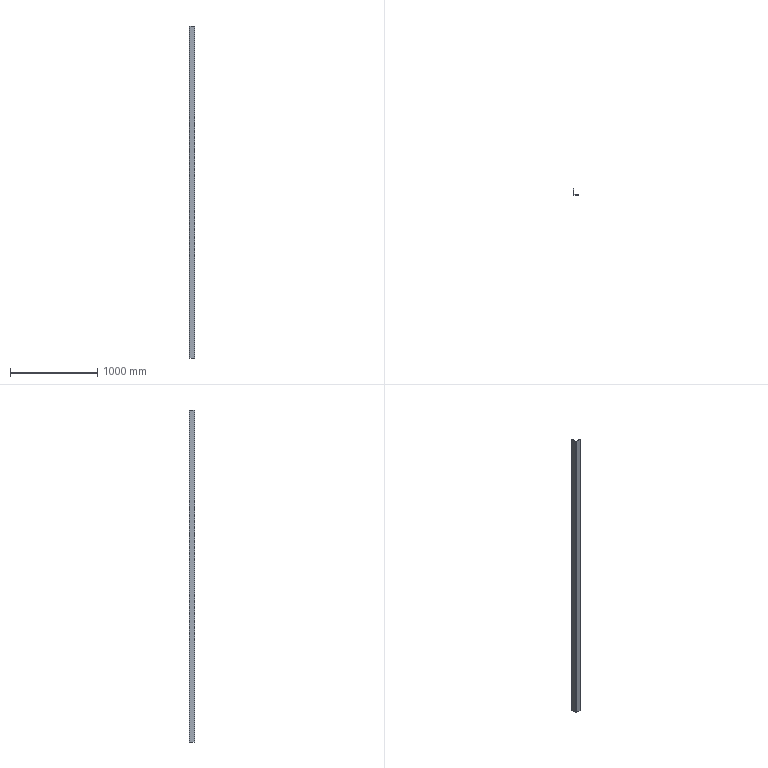Part | STEP file | BCC3 H19_9 | 1 solid | 14 faces | box 65 x 65 x 3800 mm | volume 2321993 mm3 | plane 12 | cylinder 2 | commonest cylinder face diameters 8 x1 18 x1
STEP:
#1=CARTESIAN_POINT('',(0.,0.,0.));
#2=DIRECTION('',(0.,0.,1.));
#3=DIRECTION('',(1.,0.,0.));
#4=AXIS2_PLACEMENT_3D('',#1,#2,#3);
#5=CARTESIAN_POINT('',(0.,9.,1900.));
#6=VERTEX_POINT('',#5);
#7=CARTESIAN_POINT('',(5.,9.,1900.));
#8=VERTEX_POINT('',#7);
#9=CARTESIAN_POINT('',(0.,9.,1900.));
#10=DIRECTION('',(1.,0.,0.));
#11=VECTOR('',#10,1.);
#12=LINE('',#9,#11);
#13=CARTESIAN_POINT('',(0.,9.,1900.));
#14=DIRECTION('',(0.,0.,1.));
#15=DIRECTION('',(1.,0.,0.));
#16=AXIS2_PLACEMENT_3D('',#13,#14,#15);
#17=PLANE('',#16);
#18=CARTESIAN_POINT('',(0.,0.));
#19=DIRECTION('',(1.,0.));
#20=VECTOR('',#19,1.);
#21=LINE('',#18,#20);
#22=(GEOMETRIC_REPRESENTATION_CONTEXT(2)PARAMETRIC_REPRESENTATION_CONTEXT()REPRESENTATION_CONTEXT('',''));
#23=DEFINITIONAL_REPRESENTATION('',(#21),#22);
#24=PCURVE('',#17,#23);
#25=CARTESIAN_POINT('',(9.,5.,1900.));
#26=DIRECTION('',(0.,0.,1.));
#27=DIRECTION('',(1.,0.,0.));
#28=AXIS2_PLACEMENT_3D('',#25,#26,#27);
#29=PLANE('',#28);
#30=CARTESIAN_POINT('',(-9.,4.));
#31=DIRECTION('',(1.,0.));
#32=VECTOR('',#31,1.);
#33=LINE('',#30,#32);
#34=(GEOMETRIC_REPRESENTATION_CONTEXT(2)PARAMETRIC_REPRESENTATION_CONTEXT()REPRESENTATION_CONTEXT('',''));
#35=DEFINITIONAL_REPRESENTATION('',(#33),#34);
#36=PCURVE('',#29,#35);
#37=SURFACE_CURVE('',#12,(#24,#36),.PCURVE_S1.);
#38=EDGE_CURVE('',#6,#8,#37,.T.);
#39=ORIENTED_EDGE('',*,*,#38,.F.);
#40=CARTESIAN_POINT('',(9.,0.,1900.));
#41=VERTEX_POINT('',#40);
#42=CARTESIAN_POINT('',(9.,9.,1900.));
#43=DIRECTION('',(0.,0.,1.));
#44=DIRECTION('',(-1.,0.,0.));
#45=AXIS2_PLACEMENT_3D('',#42,#43,#44);
#46=CIRCLE('',#45,9.);
#47=CARTESIAN_POINT('',(9.,0.));
#48=DIRECTION('',(-1.,0.));
#49=AXIS2_PLACEMENT_2D('',#47,#48);
#50=CIRCLE('',#49,9.);
#51=(GEOMETRIC_REPRESENTATION_CONTEXT(2)PARAMETRIC_REPRESENTATION_CONTEXT()REPRESENTATION_CONTEXT('',''));
#52=DEFINITIONAL_REPRESENTATION('',(#50),#51);
#53=PCURVE('',#17,#52);
#54=CARTESIAN_POINT('',(9.,9.,1900.));
#55=DIRECTION('',(0.,0.,-1.));
#56=DIRECTION('',(-1.,0.,0.));
#57=AXIS2_PLACEMENT_3D('',#54,#55,#56);
#58=CYLINDRICAL_SURFACE('',#57,9.);
#59=CARTESIAN_POINT('',(6.283,0.));
#60=DIRECTION('',(-1.,0.));
#61=VECTOR('',#60,1.);
#62=LINE('',#59,#61);
#63=(GEOMETRIC_REPRESENTATION_CONTEXT(2)PARAMETRIC_REPRESENTATION_CONTEXT()REPRESENTATION_CONTEXT('',''));
#64=DEFINITIONAL_REPRESENTATION('',(#62),#63);
#65=PCURVE('',#58,#64);
#66=SURFACE_CURVE('',#46,(#53,#65),.PCURVE_S1.);
#67=EDGE_CURVE('',#6,#41,#66,.T.);
#68=ORIENTED_EDGE('',*,*,#67,.T.);
#69=CARTESIAN_POINT('',(9.,5.,1900.));
#70=VERTEX_POINT('',#69);
#71=CARTESIAN_POINT('',(9.,5.,1900.));
#72=DIRECTION('',(0.,-1.,0.));
#73=VECTOR('',#72,1.);
#74=LINE('',#71,#73);
#75=CARTESIAN_POINT('',(9.,-4.));
#76=DIRECTION('',(0.,-1.));
#77=VECTOR('',#76,1.);
#78=LINE('',#75,#77);
#79=(GEOMETRIC_REPRESENTATION_CONTEXT(2)PARAMETRIC_REPRESENTATION_CONTEXT()REPRESENTATION_CONTEXT('',''));
#80=DEFINITIONAL_REPRESENTATION('',(#78),#79);
#81=PCURVE('',#17,#80);
#82=CARTESIAN_POINT('',(9.,9.,1900.));
#83=DIRECTION('',(0.,0.,1.));
#84=DIRECTION('',(1.,0.,0.));
#85=AXIS2_PLACEMENT_3D('',#82,#83,#84);
#86=PLANE('',#85);
#87=CARTESIAN_POINT('',(0.,-4.));
#88=DIRECTION('',(0.,-1.));
#89=VECTOR('',#88,1.);
#90=LINE('',#87,#89);
#91=(GEOMETRIC_REPRESENTATION_CONTEXT(2)PARAMETRIC_REPRESENTATION_CONTEXT()REPRESENTATION_CONTEXT('',''));
#92=DEFINITIONAL_REPRESENTATION('',(#90),#91);
#93=PCURVE('',#86,#92);
#94=SURFACE_CURVE('',#74,(#81,#93),.PCURVE_S1.);
#95=EDGE_CURVE('',#70,#41,#94,.T.);
#96=ORIENTED_EDGE('',*,*,#95,.F.);
#97=CARTESIAN_POINT('',(9.,9.,1900.));
#98=DIRECTION('',(0.,0.,1.));
#99=DIRECTION('',(1.,0.,0.));
#100=AXIS2_PLACEMENT_3D('',#97,#98,#99);
#101=CIRCLE('',#100,4.);
#102=CARTESIAN_POINT('',(9.,0.));
#103=DIRECTION('',(1.,0.));
#104=AXIS2_PLACEMENT_2D('',#102,#103);
#105=CIRCLE('',#104,4.);
#106=(GEOMETRIC_REPRESENTATION_CONTEXT(2)PARAMETRIC_REPRESENTATION_CONTEXT()REPRESENTATION_CONTEXT('',''));
#107=DEFINITIONAL_REPRESENTATION('',(#105),#106);
#108=PCURVE('',#17,#107);
#109=CARTESIAN_POINT('',(9.,9.,1900.));
#110=DIRECTION('',(0.,0.,-1.));
#111=DIRECTION('',(-1.,0.,0.));
#112=AXIS2_PLACEMENT_3D('',#109,#110,#111);
#113=CYLINDRICAL_SURFACE('',#112,4.);
#114=CARTESIAN_POINT('',(9.425,0.));
#115=DIRECTION('',(-1.,0.));
#116=VECTOR('',#115,1.);
#117=LINE('',#114,#116);
#118=(GEOMETRIC_REPRESENTATION_CONTEXT(2)PARAMETRIC_REPRESENTATION_CONTEXT()REPRESENTATION_CONTEXT('',''));
#119=DEFINITIONAL_REPRESENTATION('',(#117),#118);
#120=PCURVE('',#113,#119);
#121=SURFACE_CURVE('',#101,(#108,#120),.PCURVE_S1.);
#122=EDGE_CURVE('',#8,#70,#121,.T.);
#123=ORIENTED_EDGE('',*,*,#122,.F.);
#124=EDGE_LOOP('',(#39,#68,#96,#123));
#125=FACE_BOUND('',#124,.T.);
#126=ADVANCED_FACE('',(#125),#17,.T.);
#127=CARTESIAN_POINT('',(0.,65.,1900.));
#128=VERTEX_POINT('',#127);
#129=CARTESIAN_POINT('',(0.,0.,1900.));
#130=DIRECTION('',(0.,-1.,0.));
#131=VECTOR('',#130,1.);
#132=LINE('',#129,#131);
#133=CARTESIAN_POINT('',(-9.,-5.));
#134=DIRECTION('',(0.,-1.));
#135=VECTOR('',#134,1.);
#136=LINE('',#133,#135);
#137=(GEOMETRIC_REPRESENTATION_CONTEXT(2)PARAMETRIC_REPRESENTATION_CONTEXT()REPRESENTATION_CONTEXT('',''));
#138=DEFINITIONAL_REPRESENTATION('',(#136),#137);
#139=PCURVE('',#29,#138);
#140=CARTESIAN_POINT('',(0.,0.,1900.));
#141=DIRECTION('',(1.,0.,0.));
#142=DIRECTION('',(0.,0.,-1.));
#143=AXIS2_PLACEMENT_3D('',#140,#141,#142);
#144=PLANE('',#143);
#145=CARTESIAN_POINT('',(0.,0.));
#146=DIRECTION('',(0.,-1.));
#147=VECTOR('',#146,1.);
#148=LINE('',#145,#147);
#149=(GEOMETRIC_REPRESENTATION_CONTEXT(2)PARAMETRIC_REPRESENTATION_CONTEXT()REPRESENTATION_CONTEXT('',''));
#150=DEFINITIONAL_REPRESENTATION('',(#148),#149);
#151=PCURVE('',#144,#150);
#152=SURFACE_CURVE('',#132,(#139,#151),.PCURVE_S1.);
#153=EDGE_CURVE('',#128,#6,#152,.T.);
#154=ORIENTED_EDGE('',*,*,#153,.T.);
#155=ORIENTED_EDGE('',*,*,#38,.T.);
#156=CARTESIAN_POINT('',(5.,65.,1900.));
#157=VERTEX_POINT('',#156);
#158=CARTESIAN_POINT('',(5.,0.,1900.));
#159=DIRECTION('',(0.,-1.,0.));
#160=VECTOR('',#159,1.);
#161=LINE('',#158,#160);
#162=CARTESIAN_POINT('',(-4.,-5.));
#163=DIRECTION('',(0.,-1.));
#164=VECTOR('',#163,1.);
#165=LINE('',#162,#164);
#166=(GEOMETRIC_REPRESENTATION_CONTEXT(2)PARAMETRIC_REPRESENTATION_CONTEXT()REPRESENTATION_CONTEXT('',''));
#167=DEFINITIONAL_REPRESENTATION('',(#165),#166);
#168=PCURVE('',#29,#167);
#169=CARTESIAN_POINT('',(5.,0.,1900.));
#170=DIRECTION('',(1.,0.,0.));
#171=DIRECTION('',(0.,0.,-1.));
#172=AXIS2_PLACEMENT_3D('',#169,#170,#171);
#173=PLANE('',#172);
#174=CARTESIAN_POINT('',(0.,0.));
#175=DIRECTION('',(0.,-1.));
#176=VECTOR('',#175,1.);
#177=LINE('',#174,#176);
#178=(GEOMETRIC_REPRESENTATION_CONTEXT(2)PARAMETRIC_REPRESENTATION_CONTEXT()REPRESENTATION_CONTEXT('',''));
#179=DEFINITIONAL_REPRESENTATION('',(#177),#178);
#180=PCURVE('',#173,#179);
#181=SURFACE_CURVE('',#161,(#168,#180),.PCURVE_S1.);
#182=EDGE_CURVE('',#157,#8,#181,.T.);
#183=ORIENTED_EDGE('',*,*,#182,.F.);
#184=CARTESIAN_POINT('',(0.,65.,1900.));
#185=DIRECTION('',(1.,0.,0.));
#186=VECTOR('',#185,1.);
#187=LINE('',#184,#186);
#188=CARTESIAN_POINT('',(-9.,60.));
#189=DIRECTION('',(1.,0.));
#190=VECTOR('',#189,1.);
#191=LINE('',#188,#190);
#192=(GEOMETRIC_REPRESENTATION_CONTEXT(2)PARAMETRIC_REPRESENTATION_CONTEXT()REPRESENTATION_CONTEXT('',''));
#193=DEFINITIONAL_REPRESENTATION('',(#191),#192);
#194=PCURVE('',#29,#193);
#195=CARTESIAN_POINT('',(0.,65.,1900.));
#196=DIRECTION('',(0.,1.,0.));
#197=DIRECTION('',(0.,0.,1.));
#198=AXIS2_PLACEMENT_3D('',#195,#196,#197);
#199=PLANE('',#198);
#200=CARTESIAN_POINT('',(0.,0.));
#201=DIRECTION('',(0.,1.));
#202=VECTOR('',#201,1.);
#203=LINE('',#200,#202);
#204=(GEOMETRIC_REPRESENTATION_CONTEXT(2)PARAMETRIC_REPRESENTATION_CONTEXT()REPRESENTATION_CONTEXT('',''));
#205=DEFINITIONAL_REPRESENTATION('',(#203),#204);
#206=PCURVE('',#199,#205);
#207=SURFACE_CURVE('',#187,(#194,#206),.PCURVE_S1.);
#208=EDGE_CURVE('',#128,#157,#207,.T.);
#209=ORIENTED_EDGE('',*,*,#208,.F.);
#210=EDGE_LOOP('',(#154,#155,#183,#209));
#211=FACE_BOUND('',#210,.T.);
#212=ADVANCED_FACE('',(#211),#29,.T.);
#213=CARTESIAN_POINT('',(9.,0.,-1900.));
#214=VERTEX_POINT('',#213);
#215=CARTESIAN_POINT('',(9.,5.,-1900.));
#216=VERTEX_POINT('',#215);
#217=CARTESIAN_POINT('',(9.,0.,-1900.));
#218=DIRECTION('',(0.,1.,0.));
#219=VECTOR('',#218,1.);
#220=LINE('',#217,#219);
#221=CARTESIAN_POINT('',(9.,0.,-1900.));
#222=DIRECTION('',(0.,0.,-1.));
#223=DIRECTION('',(-1.,0.,0.));
#224=AXIS2_PLACEMENT_3D('',#221,#222,#223);
#225=PLANE('',#224);
#226=CARTESIAN_POINT('',(0.,0.));
#227=DIRECTION('',(0.,1.));
#228=VECTOR('',#227,1.);
#229=LINE('',#226,#228);
#230=(GEOMETRIC_REPRESENTATION_CONTEXT(2)PARAMETRIC_REPRESENTATION_CONTEXT()REPRESENTATION_CONTEXT('',''));
#231=DEFINITIONAL_REPRESENTATION('',(#229),#230);
#232=PCURVE('',#225,#231);
#233=CARTESIAN_POINT('',(5.,9.,-1900.));
#234=DIRECTION('',(0.,0.,-1.));
#235=DIRECTION('',(-1.,0.,0.));
#236=AXIS2_PLACEMENT_3D('',#233,#234,#235);
#237=PLANE('',#236);
#238=CARTESIAN_POINT('',(-4.,-9.));
#239=DIRECTION('',(0.,1.));
#240=VECTOR('',#239,1.);
#241=LINE('',#238,#240);
#242=(GEOMETRIC_REPRESENTATION_CONTEXT(2)PARAMETRIC_REPRESENTATION_CONTEXT()REPRESENTATION_CONTEXT('',''));
#243=DEFINITIONAL_REPRESENTATION('',(#241),#242);
#244=PCURVE('',#237,#243);
#245=SURFACE_CURVE('',#220,(#232,#244),.PCURVE_S1.);
#246=EDGE_CURVE('',#214,#216,#245,.T.);
#247=ORIENTED_EDGE('',*,*,#246,.F.);
#248=CARTESIAN_POINT('',(0.,9.,-1900.));
#249=VERTEX_POINT('',#248);
#250=CARTESIAN_POINT('',(9.,9.,-1900.));
#251=DIRECTION('',(0.,0.,1.));
#252=DIRECTION('',(-1.,0.,0.));
#253=AXIS2_PLACEMENT_3D('',#250,#251,#252);
#254=CIRCLE('',#253,9.);
#255=CARTESIAN_POINT('',(9.,9.));
#256=CARTESIAN_POINT('',(9.,-6.588));
#257=CARTESIAN_POINT('',(-4.5,1.206));
#258=CARTESIAN_POINT('',(-18.,9.));
#259=CARTESIAN_POINT('',(-4.5,16.794));
#260=CARTESIAN_POINT('',(9.,24.588));
#261=CARTESIAN_POINT('',(9.,9.));
#262=(BOUNDED_CURVE()B_SPLINE_CURVE(2,(#255,#256,#257,#258,#259,#260,#261),.UNSPECIFIED.,.T.,.F.)B_SPLINE_CURVE_WITH_KNOTS((1,2,2,2,2,1),(-2.094,0.,2.094,4.189,6.283,8.378),.UNSPECIFIED.)CURVE()GEOMETRIC_REPRESENTATION_ITEM()RATIONAL_B_SPLINE_CURVE((1.,0.5,1.,0.5,1.,0.5,1.))REPRESENTATION_ITEM(''));
#263=(GEOMETRIC_REPRESENTATION_CONTEXT(2)PARAMETRIC_REPRESENTATION_CONTEXT()REPRESENTATION_CONTEXT('',''));
#264=DEFINITIONAL_REPRESENTATION('',(#262),#263);
#265=PCURVE('',#225,#264);
#266=CARTESIAN_POINT('',(6.283,3800.));
#267=DIRECTION('',(-1.,0.));
#268=VECTOR('',#267,1.);
#269=LINE('',#266,#268);
#270=(GEOMETRIC_REPRESENTATION_CONTEXT(2)PARAMETRIC_REPRESENTATION_CONTEXT()REPRESENTATION_CONTEXT('',''));
#271=DEFINITIONAL_REPRESENTATION('',(#269),#270);
#272=PCURVE('',#58,#271);
#273=SURFACE_CURVE('',#254,(#265,#272),.PCURVE_S1.);
#274=EDGE_CURVE('',#249,#214,#273,.T.);
#275=ORIENTED_EDGE('',*,*,#274,.F.);
#276=CARTESIAN_POINT('',(5.,9.,-1900.));
#277=VERTEX_POINT('',#276);
#278=CARTESIAN_POINT('',(5.,9.,-1900.));
#279=DIRECTION('',(-1.,0.,0.));
#280=VECTOR('',#279,1.);
#281=LINE('',#278,#280);
#282=CARTESIAN_POINT('',(4.,9.));
#283=DIRECTION('',(1.,0.));
#284=VECTOR('',#283,1.);
#285=LINE('',#282,#284);
#286=(GEOMETRIC_REPRESENTATION_CONTEXT(2)PARAMETRIC_REPRESENTATION_CONTEXT()REPRESENTATION_CONTEXT('',''));
#287=DEFINITIONAL_REPRESENTATION('',(#285),#286);
#288=PCURVE('',#225,#287);
#289=CARTESIAN_POINT('',(9.,9.,-1900.));
#290=DIRECTION('',(0.,0.,1.));
#291=DIRECTION('',(1.,0.,0.));
#292=AXIS2_PLACEMENT_3D('',#289,#290,#291);
#293=PLANE('',#292);
#294=CARTESIAN_POINT('',(-4.,0.));
#295=DIRECTION('',(-1.,0.));
#296=VECTOR('',#295,1.);
#297=LINE('',#294,#296);
#298=(GEOMETRIC_REPRESENTATION_CONTEXT(2)PARAMETRIC_REPRESENTATION_CONTEXT()REPRESENTATION_CONTEXT('',''));
#299=DEFINITIONAL_REPRESENTATION('',(#297),#298);
#300=PCURVE('',#293,#299);
#301=SURFACE_CURVE('',#281,(#288,#300),.PCURVE_S1.);
#302=EDGE_CURVE('',#277,#249,#301,.T.);
#303=ORIENTED_EDGE('',*,*,#302,.F.);
#304=CARTESIAN_POINT('',(9.,9.,-1900.));
#305=DIRECTION('',(0.,0.,1.));
#306=DIRECTION('',(1.,0.,0.));
#307=AXIS2_PLACEMENT_3D('',#304,#305,#306);
#308=CIRCLE('',#307,4.);
#309=CARTESIAN_POINT('',(-4.,9.));
#310=CARTESIAN_POINT('',(-4.,15.928));
#311=CARTESIAN_POINT('',(2.,12.464));
#312=CARTESIAN_POINT('',(8.,9.));
#313=CARTESIAN_POINT('',(2.,5.536));
#314=CARTESIAN_POINT('',(-4.,2.072));
#315=CARTESIAN_POINT('',(-4.,9.));
#316=(BOUNDED_CURVE()B_SPLINE_CURVE(2,(#309,#310,#311,#312,#313,#314,#315),.UNSPECIFIED.,.T.,.F.)B_SPLINE_CURVE_WITH_KNOTS((1,2,2,2,2,1),(-2.094,0.,2.094,4.189,6.283,8.378),.UNSPECIFIED.)CURVE()GEOMETRIC_REPRESENTATION_ITEM()RATIONAL_B_SPLINE_CURVE((1.,0.5,1.,0.5,1.,0.5,1.))REPRESENTATION_ITEM(''));
#317=(GEOMETRIC_REPRESENTATION_CONTEXT(2)PARAMETRIC_REPRESENTATION_CONTEXT()REPRESENTATION_CONTEXT('',''));
#318=DEFINITIONAL_REPRESENTATION('',(#316),#317);
#319=PCURVE('',#225,#318);
#320=CARTESIAN_POINT('',(9.425,3800.));
#321=DIRECTION('',(-1.,0.));
#322=VECTOR('',#321,1.);
#323=LINE('',#320,#322);
#324=(GEOMETRIC_REPRESENTATION_CONTEXT(2)PARAMETRIC_REPRESENTATION_CONTEXT()REPRESENTATION_CONTEXT('',''));
#325=DEFINITIONAL_REPRESENTATION('',(#323),#324);
#326=PCURVE('',#113,#325);
#327=SURFACE_CURVE('',#308,(#319,#326),.PCURVE_S1.);
#328=EDGE_CURVE('',#277,#216,#327,.T.);
#329=ORIENTED_EDGE('',*,*,#328,.T.);
#330=EDGE_LOOP('',(#247,#275,#303,#329));
#331=FACE_BOUND('',#330,.T.);
#332=ADVANCED_FACE('',(#331),#225,.T.);
#333=CARTESIAN_POINT('',(65.,0.,-1900.));
#334=VERTEX_POINT('',#333);
#335=CARTESIAN_POINT('',(0.,0.,-1900.));
#336=DIRECTION('',(1.,0.,0.));
#337=VECTOR('',#336,1.);
#338=LINE('',#335,#337);
#339=CARTESIAN_POINT('',(5.,-9.));
#340=DIRECTION('',(-1.,0.));
#341=VECTOR('',#340,1.);
#342=LINE('',#339,#341);
#343=(GEOMETRIC_REPRESENTATION_CONTEXT(2)PARAMETRIC_REPRESENTATION_CONTEXT()REPRESENTATION_CONTEXT('',''));
#344=DEFINITIONAL_REPRESENTATION('',(#342),#343);
#345=PCURVE('',#237,#344);
#346=CARTESIAN_POINT('',(0.,0.,1900.));
#347=DIRECTION('',(0.,1.,0.));
#348=DIRECTION('',(0.,0.,1.));
#349=AXIS2_PLACEMENT_3D('',#346,#347,#348);
#350=PLANE('',#349);
#351=CARTESIAN_POINT('',(-3800.,0.));
#352=DIRECTION('',(0.,1.));
#353=VECTOR('',#352,1.);
#354=LINE('',#351,#353);
#355=(GEOMETRIC_REPRESENTATION_CONTEXT(2)PARAMETRIC_REPRESENTATION_CONTEXT()REPRESENTATION_CONTEXT('',''));
#356=DEFINITIONAL_REPRESENTATION('',(#354),#355);
#357=PCURVE('',#350,#356);
#358=SURFACE_CURVE('',#338,(#345,#357),.PCURVE_S1.);
#359=EDGE_CURVE('',#214,#334,#358,.T.);
#360=ORIENTED_EDGE('',*,*,#359,.F.);
#361=ORIENTED_EDGE('',*,*,#246,.T.);
#362=CARTESIAN_POINT('',(65.,5.,-1900.));
#363=VERTEX_POINT('',#362);
#364=CARTESIAN_POINT('',(0.,5.,-1900.));
#365=DIRECTION('',(1.,0.,0.));
#366=VECTOR('',#365,1.);
#367=LINE('',#364,#366);
#368=CARTESIAN_POINT('',(5.,-4.));
#369=DIRECTION('',(-1.,0.));
#370=VECTOR('',#369,1.);
#371=LINE('',#368,#370);
#372=(GEOMETRIC_REPRESENTATION_CONTEXT(2)PARAMETRIC_REPRESENTATION_CONTEXT()REPRESENTATION_CONTEXT('',''));
#373=DEFINITIONAL_REPRESENTATION('',(#371),#372);
#374=PCURVE('',#237,#373);
#375=CARTESIAN_POINT('',(0.,5.,1900.));
#376=DIRECTION('',(0.,1.,0.));
#377=DIRECTION('',(0.,0.,1.));
#378=AXIS2_PLACEMENT_3D('',#375,#376,#377);
#379=PLANE('',#378);
#380=CARTESIAN_POINT('',(-3800.,0.));
#381=DIRECTION('',(0.,1.));
#382=VECTOR('',#381,1.);
#383=LINE('',#380,#382);
#384=(GEOMETRIC_REPRESENTATION_CONTEXT(2)PARAMETRIC_REPRESENTATION_CONTEXT()REPRESENTATION_CONTEXT('',''));
#385=DEFINITIONAL_REPRESENTATION('',(#383),#384);
#386=PCURVE('',#379,#385);
#387=SURFACE_CURVE('',#367,(#374,#386),.PCURVE_S1.);
#388=EDGE_CURVE('',#216,#363,#387,.T.);
#389=ORIENTED_EDGE('',*,*,#388,.T.);
#390=CARTESIAN_POINT('',(65.,5.,-1900.));
#391=DIRECTION('',(0.,-1.,0.));
#392=VECTOR('',#391,1.);
#393=LINE('',#390,#392);
#394=CARTESIAN_POINT('',(-60.,-4.));
#395=DIRECTION('',(0.,-1.));
#396=VECTOR('',#395,1.);
#397=LINE('',#394,#396);
#398=(GEOMETRIC_REPRESENTATION_CONTEXT(2)PARAMETRIC_REPRESENTATION_CONTEXT()REPRESENTATION_CONTEXT('',''));
#399=DEFINITIONAL_REPRESENTATION('',(#397),#398);
#400=PCURVE('',#237,#399);
#401=CARTESIAN_POINT('',(65.,5.,1900.));
#402=DIRECTION('',(1.,0.,0.));
#403=DIRECTION('',(0.,0.,-1.));
#404=AXIS2_PLACEMENT_3D('',#401,#402,#403);
#405=PLANE('',#404);
#406=CARTESIAN_POINT('',(3800.,0.));
#407=DIRECTION('',(0.,-1.));
#408=VECTOR('',#407,1.);
#409=LINE('',#406,#408);
#410=(GEOMETRIC_REPRESENTATION_CONTEXT(2)PARAMETRIC_REPRESENTATION_CONTEXT()REPRESENTATION_CONTEXT('',''));
#411=DEFINITIONAL_REPRESENTATION('',(#409),#410);
#412=PCURVE('',#405,#411);
#413=SURFACE_CURVE('',#393,(#400,#412),.PCURVE_S1.);
#414=EDGE_CURVE('',#363,#334,#413,.T.);
#415=ORIENTED_EDGE('',*,*,#414,.T.);
#416=EDGE_LOOP('',(#360,#361,#389,#415));
#417=FACE_BOUND('',#416,.T.);
#418=ADVANCED_FACE('',(#417),#237,.T.);
#419=ORIENTED_EDGE('',*,*,#359,.T.);
#420=CARTESIAN_POINT('',(65.,0.,1900.));
#421=VERTEX_POINT('',#420);
#422=CARTESIAN_POINT('',(65.,0.,1900.));
#423=DIRECTION('',(0.,0.,-1.));
#424=VECTOR('',#423,1.);
#425=LINE('',#422,#424);
#426=CARTESIAN_POINT('',(0.,65.));
#427=DIRECTION('',(-1.,0.));
#428=VECTOR('',#427,1.);
#429=LINE('',#426,#428);
#430=(GEOMETRIC_REPRESENTATION_CONTEXT(2)PARAMETRIC_REPRESENTATION_CONTEXT()REPRESENTATION_CONTEXT('',''));
#431=DEFINITIONAL_REPRESENTATION('',(#429),#430);
#432=PCURVE('',#350,#431);
#433=CARTESIAN_POINT('',(0.,-5.));
#434=DIRECTION('',(1.,0.));
#435=VECTOR('',#434,1.);
#436=LINE('',#433,#435);
#437=(GEOMETRIC_REPRESENTATION_CONTEXT(2)PARAMETRIC_REPRESENTATION_CONTEXT()REPRESENTATION_CONTEXT('',''));
#438=DEFINITIONAL_REPRESENTATION('',(#436),#437);
#439=PCURVE('',#405,#438);
#440=SURFACE_CURVE('',#425,(#432,#439),.PCURVE_S1.);
#441=EDGE_CURVE('',#421,#334,#440,.T.);
#442=ORIENTED_EDGE('',*,*,#441,.F.);
#443=CARTESIAN_POINT('',(0.,0.,1900.));
#444=DIRECTION('',(1.,0.,0.));
#445=VECTOR('',#444,1.);
#446=LINE('',#443,#445);
#447=CARTESIAN_POINT('',(0.,0.));
#448=DIRECTION('',(0.,1.));
#449=VECTOR('',#448,1.);
#450=LINE('',#447,#449);
#451=(GEOMETRIC_REPRESENTATION_CONTEXT(2)PARAMETRIC_REPRESENTATION_CONTEXT()REPRESENTATION_CONTEXT('',''));
#452=DEFINITIONAL_REPRESENTATION('',(#450),#451);
#453=PCURVE('',#350,#452);
#454=CARTESIAN_POINT('',(-9.,-9.));
#455=DIRECTION('',(1.,0.));
#456=VECTOR('',#455,1.);
#457=LINE('',#454,#456);
#458=(GEOMETRIC_REPRESENTATION_CONTEXT(2)PARAMETRIC_REPRESENTATION_CONTEXT()REPRESENTATION_CONTEXT('',''));
#459=DEFINITIONAL_REPRESENTATION('',(#457),#458);
#460=PCURVE('',#86,#459);
#461=SURFACE_CURVE('',#446,(#453,#460),.PCURVE_S1.);
#462=EDGE_CURVE('',#41,#421,#461,.T.);
#463=ORIENTED_EDGE('',*,*,#462,.F.);
#464=CARTESIAN_POINT('',(9.,0.,1900.));
#465=DIRECTION('',(0.,0.,-1.));
#466=VECTOR('',#465,1.);
#467=LINE('',#464,#466);
#468=CARTESIAN_POINT('',(0.,9.));
#469=DIRECTION('',(-1.,0.));
#470=VECTOR('',#469,1.);
#471=LINE('',#468,#470);
#472=(GEOMETRIC_REPRESENTATION_CONTEXT(2)PARAMETRIC_REPRESENTATION_CONTEXT()REPRESENTATION_CONTEXT('',''));
#473=DEFINITIONAL_REPRESENTATION('',(#471),#472);
#474=PCURVE('',#350,#473);
#475=CARTESIAN_POINT('',(4.712,0.));
#476=DIRECTION('',(0.,1.));
#477=VECTOR('',#476,1.);
#478=LINE('',#475,#477);
#479=(GEOMETRIC_REPRESENTATION_CONTEXT(2)PARAMETRIC_REPRESENTATION_CONTEXT()REPRESENTATION_CONTEXT('',''));
#480=DEFINITIONAL_REPRESENTATION('',(#478),#479);
#481=PCURVE('',#58,#480);
#482=SURFACE_CURVE('',#467,(#474,#481),.PCURVE_S1.);
#483=EDGE_CURVE('',#41,#214,#482,.T.);
#484=ORIENTED_EDGE('',*,*,#483,.T.);
#485=EDGE_LOOP('',(#419,#442,#463,#484));
#486=FACE_BOUND('',#485,.T.);
#487=ADVANCED_FACE('',(#486),#350,.F.);
#488=ORIENTED_EDGE('',*,*,#414,.F.);
#489=CARTESIAN_POINT('',(65.,5.,1900.));
#490=VERTEX_POINT('',#489);
#491=CARTESIAN_POINT('',(65.,5.,1900.));
#492=DIRECTION('',(0.,0.,-1.));
#493=VECTOR('',#492,1.);
#494=LINE('',#491,#493);
#495=CARTESIAN_POINT('',(0.,0.));
#496=DIRECTION('',(1.,0.));
#497=VECTOR('',#496,1.);
#498=LINE('',#495,#497);
#499=(GEOMETRIC_REPRESENTATION_CONTEXT(2)PARAMETRIC_REPRESENTATION_CONTEXT()REPRESENTATION_CONTEXT('',''));
#500=DEFINITIONAL_REPRESENTATION('',(#498),#499);
#501=PCURVE('',#405,#500);
#502=CARTESIAN_POINT('',(0.,65.));
#503=DIRECTION('',(-1.,0.));
#504=VECTOR('',#503,1.);
#505=LINE('',#502,#504);
#506=(GEOMETRIC_REPRESENTATION_CONTEXT(2)PARAMETRIC_REPRESENTATION_CONTEXT()REPRESENTATION_CONTEXT('',''));
#507=DEFINITIONAL_REPRESENTATION('',(#505),#506);
#508=PCURVE('',#379,#507);
#509=SURFACE_CURVE('',#494,(#501,#508),.PCURVE_S1.);
#510=EDGE_CURVE('',#490,#363,#509,.T.);
#511=ORIENTED_EDGE('',*,*,#510,.F.);
#512=CARTESIAN_POINT('',(65.,5.,1900.));
#513=DIRECTION('',(0.,-1.,0.));
#514=VECTOR('',#513,1.);
#515=LINE('',#512,#514);
#516=CARTESIAN_POINT('',(0.,0.));
#517=DIRECTION('',(0.,-1.));
#518=VECTOR('',#517,1.);
#519=LINE('',#516,#518);
#520=(GEOMETRIC_REPRESENTATION_CONTEXT(2)PARAMETRIC_REPRESENTATION_CONTEXT()REPRESENTATION_CONTEXT('',''));
#521=DEFINITIONAL_REPRESENTATION('',(#519),#520);
#522=PCURVE('',#405,#521);
#523=CARTESIAN_POINT('',(56.,-4.));
#524=DIRECTION('',(0.,-1.));
#525=VECTOR('',#524,1.);
#526=LINE('',#523,#525);
#527=(GEOMETRIC_REPRESENTATION_CONTEXT(2)PARAMETRIC_REPRESENTATION_CONTEXT()REPRESENTATION_CONTEXT('',''));
#528=DEFINITIONAL_REPRESENTATION('',(#526),#527);
#529=PCURVE('',#86,#528);
#530=SURFACE_CURVE('',#515,(#522,#529),.PCURVE_S1.);
#531=EDGE_CURVE('',#490,#421,#530,.T.);
#532=ORIENTED_EDGE('',*,*,#531,.T.);
#533=ORIENTED_EDGE('',*,*,#441,.T.);
#534=EDGE_LOOP('',(#488,#511,#532,#533));
#535=FACE_BOUND('',#534,.T.);
#536=ADVANCED_FACE('',(#535),#405,.T.);
#537=ORIENTED_EDGE('',*,*,#388,.F.);
#538=CARTESIAN_POINT('',(9.,5.,1900.));
#539=DIRECTION('',(0.,0.,-1.));
#540=VECTOR('',#539,1.);
#541=LINE('',#538,#540);
#542=CARTESIAN_POINT('',(0.,9.));
#543=DIRECTION('',(-1.,0.));
#544=VECTOR('',#543,1.);
#545=LINE('',#542,#544);
#546=(GEOMETRIC_REPRESENTATION_CONTEXT(2)PARAMETRIC_REPRESENTATION_CONTEXT()REPRESENTATION_CONTEXT('',''));
#547=DEFINITIONAL_REPRESENTATION('',(#545),#546);
#548=PCURVE('',#379,#547);
#549=CARTESIAN_POINT('',(4.712,0.));
#550=DIRECTION('',(0.,1.));
#551=VECTOR('',#550,1.);
#552=LINE('',#549,#551);
#553=(GEOMETRIC_REPRESENTATION_CONTEXT(2)PARAMETRIC_REPRESENTATION_CONTEXT()REPRESENTATION_CONTEXT('',''));
#554=DEFINITIONAL_REPRESENTATION('',(#552),#553);
#555=PCURVE('',#113,#554);
#556=SURFACE_CURVE('',#541,(#548,#555),.PCURVE_S1.);
#557=EDGE_CURVE('',#70,#216,#556,.T.);
#558=ORIENTED_EDGE('',*,*,#557,.F.);
#559=CARTESIAN_POINT('',(0.,5.,1900.));
#560=DIRECTION('',(1.,0.,0.));
#561=VECTOR('',#560,1.);
#562=LINE('',#559,#561);
#563=CARTESIAN_POINT('',(0.,0.));
#564=DIRECTION('',(0.,1.));
#565=VECTOR('',#564,1.);
#566=LINE('',#563,#565);
#567=(GEOMETRIC_REPRESENTATION_CONTEXT(2)PARAMETRIC_REPRESENTATION_CONTEXT()REPRESENTATION_CONTEXT('',''));
#568=DEFINITIONAL_REPRESENTATION('',(#566),#567);
#569=PCURVE('',#379,#568);
#570=CARTESIAN_POINT('',(-9.,-4.));
#571=DIRECTION('',(1.,0.));
#572=VECTOR('',#571,1.);
#573=LINE('',#570,#572);
#574=(GEOMETRIC_REPRESENTATION_CONTEXT(2)PARAMETRIC_REPRESENTATION_CONTEXT()REPRESENTATION_CONTEXT('',''));
#575=DEFINITIONAL_REPRESENTATION('',(#573),#574);
#576=PCURVE('',#86,#575);
#577=SURFACE_CURVE('',#562,(#569,#576),.PCURVE_S1.);
#578=EDGE_CURVE('',#70,#490,#577,.T.);
#579=ORIENTED_EDGE('',*,*,#578,.T.);
#580=ORIENTED_EDGE('',*,*,#510,.T.);
#581=EDGE_LOOP('',(#537,#558,#579,#580));
#582=FACE_BOUND('',#581,.T.);
#583=ADVANCED_FACE('',(#582),#379,.T.);
#584=ORIENTED_EDGE('',*,*,#557,.F.);
#585=ORIENTED_EDGE('',*,*,#122,.F.);
#586=CARTESIAN_POINT('',(5.,9.,1900.));
#587=DIRECTION('',(0.,0.,-1.));
#588=VECTOR('',#587,1.);
#589=LINE('',#586,#588);
#590=CARTESIAN_POINT('',(6.283,0.));
#591=DIRECTION('',(0.,1.));
#592=VECTOR('',#591,1.);
#593=LINE('',#590,#592);
#594=(GEOMETRIC_REPRESENTATION_CONTEXT(2)PARAMETRIC_REPRESENTATION_CONTEXT()REPRESENTATION_CONTEXT('',''));
#595=DEFINITIONAL_REPRESENTATION('',(#593),#594);
#596=PCURVE('',#113,#595);
#597=CARTESIAN_POINT('',(0.,9.));
#598=DIRECTION('',(1.,0.));
#599=VECTOR('',#598,1.);
#600=LINE('',#597,#599);
#601=(GEOMETRIC_REPRESENTATION_CONTEXT(2)PARAMETRIC_REPRESENTATION_CONTEXT()REPRESENTATION_CONTEXT('',''));
#602=DEFINITIONAL_REPRESENTATION('',(#600),#601);
#603=PCURVE('',#173,#602);
#604=SURFACE_CURVE('',#589,(#596,#603),.PCURVE_S1.);
#605=EDGE_CURVE('',#8,#277,#604,.T.);
#606=ORIENTED_EDGE('',*,*,#605,.T.);
#607=ORIENTED_EDGE('',*,*,#328,.T.);
#608=EDGE_LOOP('',(#584,#585,#606,#607));
#609=FACE_BOUND('',#608,.F.);
#610=ADVANCED_FACE('',(#609),#113,.F.);
#611=CARTESIAN_POINT('',(5.,65.,-1900.));
#612=VERTEX_POINT('',#611);
#613=CARTESIAN_POINT('',(5.,0.,-1900.));
#614=DIRECTION('',(0.,-1.,0.));
#615=VECTOR('',#614,1.);
#616=LINE('',#613,#615);
#617=CARTESIAN_POINT('',(3800.,0.));
#618=DIRECTION('',(0.,-1.));
#619=VECTOR('',#618,1.);
#620=LINE('',#617,#619);
#621=(GEOMETRIC_REPRESENTATION_CONTEXT(2)PARAMETRIC_REPRESENTATION_CONTEXT()REPRESENTATION_CONTEXT('',''));
#622=DEFINITIONAL_REPRESENTATION('',(#620),#621);
#623=PCURVE('',#173,#622);
#624=CARTESIAN_POINT('',(-4.,-9.));
#625=DIRECTION('',(0.,-1.));
#626=VECTOR('',#625,1.);
#627=LINE('',#624,#626);
#628=(GEOMETRIC_REPRESENTATION_CONTEXT(2)PARAMETRIC_REPRESENTATION_CONTEXT()REPRESENTATION_CONTEXT('',''));
#629=DEFINITIONAL_REPRESENTATION('',(#627),#628);
#630=PCURVE('',#293,#629);
#631=SURFACE_CURVE('',#616,(#623,#630),.PCURVE_S1.);
#632=EDGE_CURVE('',#612,#277,#631,.T.);
#633=ORIENTED_EDGE('',*,*,#632,.F.);
#634=CARTESIAN_POINT('',(5.,65.,1900.));
#635=DIRECTION('',(0.,0.,-1.));
#636=VECTOR('',#635,1.);
#637=LINE('',#634,#636);
#638=CARTESIAN_POINT('',(0.,65.));
#639=DIRECTION('',(1.,0.));
#640=VECTOR('',#639,1.);
#641=LINE('',#638,#640);
#642=(GEOMETRIC_REPRESENTATION_CONTEXT(2)PARAMETRIC_REPRESENTATION_CONTEXT()REPRESENTATION_CONTEXT('',''));
#643=DEFINITIONAL_REPRESENTATION('',(#641),#642);
#644=PCURVE('',#173,#643);
#645=CARTESIAN_POINT('',(0.,5.));
#646=DIRECTION('',(-1.,0.));
#647=VECTOR('',#646,1.);
#648=LINE('',#645,#647);
#649=(GEOMETRIC_REPRESENTATION_CONTEXT(2)PARAMETRIC_REPRESENTATION_CONTEXT()REPRESENTATION_CONTEXT('',''));
#650=DEFINITIONAL_REPRESENTATION('',(#648),#649);
#651=PCURVE('',#199,#650);
#652=SURFACE_CURVE('',#637,(#644,#651),.PCURVE_S1.);
#653=EDGE_CURVE('',#157,#612,#652,.T.);
#654=ORIENTED_EDGE('',*,*,#653,.F.);
#655=ORIENTED_EDGE('',*,*,#182,.T.);
#656=ORIENTED_EDGE('',*,*,#605,.T.);
#657=EDGE_LOOP('',(#633,#654,#655,#656));
#658=FACE_BOUND('',#657,.T.);
#659=ADVANCED_FACE('',(#658),#173,.T.);
#660=CARTESIAN_POINT('',(0.,65.,-1900.));
#661=VERTEX_POINT('',#660);
#662=CARTESIAN_POINT('',(0.,65.,-1900.));
#663=DIRECTION('',(1.,0.,0.));
#664=VECTOR('',#663,1.);
#665=LINE('',#662,#664);
#666=CARTESIAN_POINT('',(-3800.,0.));
#667=DIRECTION('',(0.,1.));
#668=VECTOR('',#667,1.);
#669=LINE('',#666,#668);
#670=(GEOMETRIC_REPRESENTATION_CONTEXT(2)PARAMETRIC_REPRESENTATION_CONTEXT()REPRESENTATION_CONTEXT('',''));
#671=DEFINITIONAL_REPRESENTATION('',(#669),#670);
#672=PCURVE('',#199,#671);
#673=CARTESIAN_POINT('',(-9.,56.));
#674=DIRECTION('',(1.,0.));
#675=VECTOR('',#674,1.);
#676=LINE('',#673,#675);
#677=(GEOMETRIC_REPRESENTATION_CONTEXT(2)PARAMETRIC_REPRESENTATION_CONTEXT()REPRESENTATION_CONTEXT('',''));
#678=DEFINITIONAL_REPRESENTATION('',(#676),#677);
#679=PCURVE('',#293,#678);
#680=SURFACE_CURVE('',#665,(#672,#679),.PCURVE_S1.);
#681=EDGE_CURVE('',#661,#612,#680,.T.);
#682=ORIENTED_EDGE('',*,*,#681,.F.);
#683=CARTESIAN_POINT('',(0.,65.,1900.));
#684=DIRECTION('',(0.,0.,-1.));
#685=VECTOR('',#684,1.);
#686=LINE('',#683,#685);
#687=CARTESIAN_POINT('',(0.,0.));
#688=DIRECTION('',(-1.,0.));
#689=VECTOR('',#688,1.);
#690=LINE('',#687,#689);
#691=(GEOMETRIC_REPRESENTATION_CONTEXT(2)PARAMETRIC_REPRESENTATION_CONTEXT()REPRESENTATION_CONTEXT('',''));
#692=DEFINITIONAL_REPRESENTATION('',(#690),#691);
#693=PCURVE('',#199,#692);
#694=CARTESIAN_POINT('',(0.,65.));
#695=DIRECTION('',(1.,0.));
#696=VECTOR('',#695,1.);
#697=LINE('',#694,#696);
#698=(GEOMETRIC_REPRESENTATION_CONTEXT(2)PARAMETRIC_REPRESENTATION_CONTEXT()REPRESENTATION_CONTEXT('',''));
#699=DEFINITIONAL_REPRESENTATION('',(#697),#698);
#700=PCURVE('',#144,#699);
#701=SURFACE_CURVE('',#686,(#693,#700),.PCURVE_S1.);
#702=EDGE_CURVE('',#128,#661,#701,.T.);
#703=ORIENTED_EDGE('',*,*,#702,.F.);
#704=ORIENTED_EDGE('',*,*,#208,.T.);
#705=ORIENTED_EDGE('',*,*,#653,.T.);
#706=EDGE_LOOP('',(#682,#703,#704,#705));
#707=FACE_BOUND('',#706,.T.);
#708=ADVANCED_FACE('',(#707),#199,.T.);
#709=CARTESIAN_POINT('',(0.,0.,-1900.));
#710=DIRECTION('',(0.,-1.,0.));
#711=VECTOR('',#710,1.);
#712=LINE('',#709,#711);
#713=CARTESIAN_POINT('',(3800.,0.));
#714=DIRECTION('',(0.,-1.));
#715=VECTOR('',#714,1.);
#716=LINE('',#713,#715);
#717=(GEOMETRIC_REPRESENTATION_CONTEXT(2)PARAMETRIC_REPRESENTATION_CONTEXT()REPRESENTATION_CONTEXT('',''));
#718=DEFINITIONAL_REPRESENTATION('',(#716),#717);
#719=PCURVE('',#144,#718);
#720=CARTESIAN_POINT('',(-9.,-9.));
#721=DIRECTION('',(0.,-1.));
#722=VECTOR('',#721,1.);
#723=LINE('',#720,#722);
#724=(GEOMETRIC_REPRESENTATION_CONTEXT(2)PARAMETRIC_REPRESENTATION_CONTEXT()REPRESENTATION_CONTEXT('',''));
#725=DEFINITIONAL_REPRESENTATION('',(#723),#724);
#726=PCURVE('',#293,#725);
#727=SURFACE_CURVE('',#712,(#719,#726),.PCURVE_S1.);
#728=EDGE_CURVE('',#661,#249,#727,.T.);
#729=ORIENTED_EDGE('',*,*,#728,.T.);
#730=CARTESIAN_POINT('',(0.,9.,1900.));
#731=DIRECTION('',(0.,0.,-1.));
#732=VECTOR('',#731,1.);
#733=LINE('',#730,#732);
#734=CARTESIAN_POINT('',(0.,9.));
#735=DIRECTION('',(1.,0.));
#736=VECTOR('',#735,1.);
#737=LINE('',#734,#736);
#738=(GEOMETRIC_REPRESENTATION_CONTEXT(2)PARAMETRIC_REPRESENTATION_CONTEXT()REPRESENTATION_CONTEXT('',''));
#739=DEFINITIONAL_REPRESENTATION('',(#737),#738);
#740=PCURVE('',#144,#739);
#741=CARTESIAN_POINT('',(6.283,0.));
#742=DIRECTION('',(0.,1.));
#743=VECTOR('',#742,1.);
#744=LINE('',#741,#743);
#745=(GEOMETRIC_REPRESENTATION_CONTEXT(2)PARAMETRIC_REPRESENTATION_CONTEXT()REPRESENTATION_CONTEXT('',''));
#746=DEFINITIONAL_REPRESENTATION('',(#744),#745);
#747=PCURVE('',#58,#746);
#748=SURFACE_CURVE('',#733,(#740,#747),.PCURVE_S1.);
#749=EDGE_CURVE('',#6,#249,#748,.T.);
#750=ORIENTED_EDGE('',*,*,#749,.F.);
#751=ORIENTED_EDGE('',*,*,#153,.F.);
#752=ORIENTED_EDGE('',*,*,#702,.T.);
#753=EDGE_LOOP('',(#729,#750,#751,#752));
#754=FACE_BOUND('',#753,.T.);
#755=ADVANCED_FACE('',(#754),#144,.F.);
#756=ORIENTED_EDGE('',*,*,#274,.T.);
#757=ORIENTED_EDGE('',*,*,#483,.F.);
#758=ORIENTED_EDGE('',*,*,#67,.F.);
#759=ORIENTED_EDGE('',*,*,#749,.T.);
#760=EDGE_LOOP('',(#756,#757,#758,#759));
#761=FACE_BOUND('',#760,.T.);
#762=ADVANCED_FACE('',(#761),#58,.T.);
#763=ORIENTED_EDGE('',*,*,#462,.T.);
#764=ORIENTED_EDGE('',*,*,#531,.F.);
#765=ORIENTED_EDGE('',*,*,#578,.F.);
#766=ORIENTED_EDGE('',*,*,#95,.T.);
#767=EDGE_LOOP('',(#763,#764,#765,#766));
#768=FACE_BOUND('',#767,.T.);
#769=ADVANCED_FACE('',(#768),#86,.T.);
#770=ORIENTED_EDGE('',*,*,#632,.T.);
#771=ORIENTED_EDGE('',*,*,#302,.T.);
#772=ORIENTED_EDGE('',*,*,#728,.F.);
#773=ORIENTED_EDGE('',*,*,#681,.T.);
#774=EDGE_LOOP('',(#770,#771,#772,#773));
#775=FACE_BOUND('',#774,.T.);
#776=ADVANCED_FACE('',(#775),#293,.F.);
#777=CLOSED_SHELL('',(#126,#212,#332,#418,#487,#536,#583,#610,#659,#708,#755,#762,#769,#776));
#778=MANIFOLD_SOLID_BREP('',#777);
#779=(LENGTH_UNIT()NAMED_UNIT(*)SI_UNIT(.MILLI.,.METRE.));
#780=UNCERTAINTY_MEASURE_WITH_UNIT(LENGTH_MEASURE(0.0000001),#779,'','');
#781=(NAMED_UNIT(*)PLANE_ANGLE_UNIT()SI_UNIT($,.RADIAN.));
#782=(NAMED_UNIT(*)SI_UNIT($,.STERADIAN.)SOLID_ANGLE_UNIT());
#783=(GEOMETRIC_REPRESENTATION_CONTEXT(3)GLOBAL_UNCERTAINTY_ASSIGNED_CONTEXT((#780))GLOBAL_UNIT_ASSIGNED_CONTEXT((#779,#781,#782))REPRESENTATION_CONTEXT('',''));
#784=ADVANCED_BREP_SHAPE_REPRESENTATION('',(#4,#778),#783);